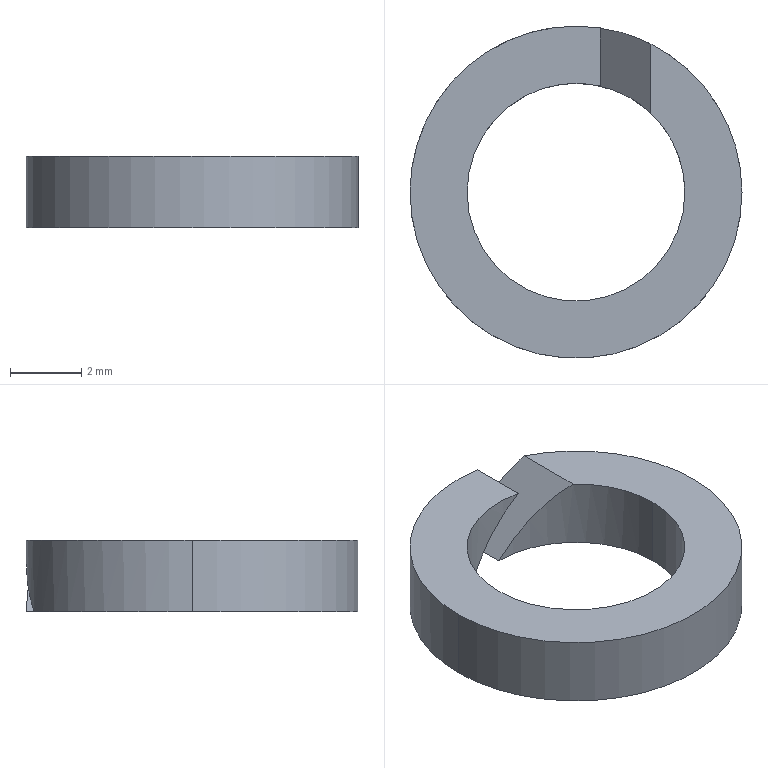Part | STEP file | 921271103 | 1 solid | 10 faces | box 9.3 x 9.3 x 2 mm | volume 72.768 mm3 | cylinder 6 | plane 4 | commonest cylinder face diameters 6.1 x3 9.3 x3
STEP:
#1=CARTESIAN_POINT('',(2.1,4.149,2.));
#2=VERTEX_POINT('',#1);
#3=CARTESIAN_POINT('',(4.65,0.,2.));
#4=VERTEX_POINT('',#3);
#5=CARTESIAN_POINT('',(0.,0.,2.));
#6=DIRECTION('',(0.,0.,-1.));
#7=DIRECTION('',(-1.,0.,0.));
#8=AXIS2_PLACEMENT_3D('',#5,#6,#7);
#9=CIRCLE('',#8,4.65);
#10=EDGE_CURVE('',#2,#4,#9,.T.);
#11=ORIENTED_EDGE('',*,*,#10,.T.);
#12=CARTESIAN_POINT('',(4.65,0.,0.));
#13=VERTEX_POINT('',#12);
#14=CARTESIAN_POINT('',(4.65,0.,2.));
#15=DIRECTION('',(0.,0.,-1.));
#16=VECTOR('',#15,1000.);
#17=LINE('',#14,#16);
#18=EDGE_CURVE('',#4,#13,#17,.T.);
#19=ORIENTED_EDGE('',*,*,#18,.T.);
#20=CARTESIAN_POINT('',(0.,4.65,0.));
#21=VERTEX_POINT('',#20);
#22=CARTESIAN_POINT('',(0.,0.,0.));
#23=DIRECTION('',(0.,0.,1.));
#24=DIRECTION('',(-1.,0.,0.));
#25=AXIS2_PLACEMENT_3D('',#22,#23,#24);
#26=CIRCLE('',#25,4.65);
#27=EDGE_CURVE('',#13,#21,#26,.T.);
#28=ORIENTED_EDGE('',*,*,#27,.T.);
#29=CARTESIAN_POINT('',(0.,4.65,0.));
#30=CARTESIAN_POINT('',(0.733,4.65,0.6981));
#31=CARTESIAN_POINT('',(1.446,4.48,1.377));
#32=CARTESIAN_POINT('',(2.1,4.149,2.));
#33=(BOUNDED_CURVE()B_SPLINE_CURVE(3,(#29,#30,#31,#32),.UNSPECIFIED.,.F.,.F.)B_SPLINE_CURVE_WITH_KNOTS((4,4),(1.571,2.039),.UNSPECIFIED.)CURVE()GEOMETRIC_REPRESENTATION_ITEM()RATIONAL_B_SPLINE_CURVE((1.,0.9818,0.9818,1.))REPRESENTATION_ITEM(''));
#34=EDGE_CURVE('',#21,#2,#33,.T.);
#35=ORIENTED_EDGE('',*,*,#34,.T.);
#36=EDGE_LOOP('',(#11,#19,#28,#35));
#37=FACE_OUTER_BOUND('',#36,.T.);
#38=CARTESIAN_POINT('',(0.,0.,2.));
#39=DIRECTION('',(0.,0.,-1.));
#40=DIRECTION('',(-1.,0.,0.));
#41=AXIS2_PLACEMENT_3D('',#38,#39,#40);
#42=CYLINDRICAL_SURFACE('',#41,4.65);
#43=ADVANCED_FACE('',(#37),#42,.T.);
#44=ORIENTED_EDGE('',*,*,#18,.F.);
#45=CARTESIAN_POINT('',(-4.65,0.,2.));
#46=VERTEX_POINT('',#45);
#47=CARTESIAN_POINT('',(0.,0.,2.));
#48=DIRECTION('',(0.,0.,-1.));
#49=DIRECTION('',(-1.,0.,0.));
#50=AXIS2_PLACEMENT_3D('',#47,#48,#49);
#51=CIRCLE('',#50,4.65);
#52=EDGE_CURVE('',#4,#46,#51,.T.);
#53=ORIENTED_EDGE('',*,*,#52,.T.);
#54=CARTESIAN_POINT('',(-4.65,0.,0.));
#55=VERTEX_POINT('',#54);
#56=CARTESIAN_POINT('',(-4.65,0.,2.));
#57=DIRECTION('',(0.,0.,-1.));
#58=VECTOR('',#57,1000.);
#59=LINE('',#56,#58);
#60=EDGE_CURVE('',#46,#55,#59,.T.);
#61=ORIENTED_EDGE('',*,*,#60,.T.);
#62=CARTESIAN_POINT('',(0.,0.,0.));
#63=DIRECTION('',(0.,0.,1.));
#64=DIRECTION('',(-1.,0.,0.));
#65=AXIS2_PLACEMENT_3D('',#62,#63,#64);
#66=CIRCLE('',#65,4.65);
#67=EDGE_CURVE('',#55,#13,#66,.T.);
#68=ORIENTED_EDGE('',*,*,#67,.T.);
#69=EDGE_LOOP('',(#44,#53,#61,#68));
#70=FACE_OUTER_BOUND('',#69,.T.);
#71=CARTESIAN_POINT('',(0.,0.,2.));
#72=DIRECTION('',(0.,0.,-1.));
#73=DIRECTION('',(-1.,0.,0.));
#74=AXIS2_PLACEMENT_3D('',#71,#72,#73);
#75=CYLINDRICAL_SURFACE('',#74,4.65);
#76=ADVANCED_FACE('',(#70),#75,.T.);
#77=CARTESIAN_POINT('',(-3.05,0.,2.));
#78=VERTEX_POINT('',#77);
#79=CARTESIAN_POINT('',(3.05,0.,2.));
#80=VERTEX_POINT('',#79);
#81=CARTESIAN_POINT('',(0.,0.,2.));
#82=DIRECTION('',(0.,0.,1.));
#83=DIRECTION('',(-1.,0.,0.));
#84=AXIS2_PLACEMENT_3D('',#81,#82,#83);
#85=CIRCLE('',#84,3.05);
#86=EDGE_CURVE('',#78,#80,#85,.T.);
#87=ORIENTED_EDGE('',*,*,#86,.T.);
#88=CARTESIAN_POINT('',(3.05,0.,0.));
#89=VERTEX_POINT('',#88);
#90=CARTESIAN_POINT('',(3.05,0.,2.));
#91=DIRECTION('',(0.,0.,-1.));
#92=VECTOR('',#91,1000.);
#93=LINE('',#90,#92);
#94=EDGE_CURVE('',#80,#89,#93,.T.);
#95=ORIENTED_EDGE('',*,*,#94,.T.);
#96=CARTESIAN_POINT('',(-3.05,0.,0.));
#97=VERTEX_POINT('',#96);
#98=CARTESIAN_POINT('',(0.,0.,0.));
#99=DIRECTION('',(0.,0.,1.));
#100=DIRECTION('',(-1.,0.,0.));
#101=AXIS2_PLACEMENT_3D('',#98,#99,#100);
#102=CIRCLE('',#101,3.05);
#103=EDGE_CURVE('',#97,#89,#102,.T.);
#104=ORIENTED_EDGE('',*,*,#103,.F.);
#105=CARTESIAN_POINT('',(-3.05,0.,2.));
#106=DIRECTION('',(0.,0.,-1.));
#107=VECTOR('',#106,1000.);
#108=LINE('',#105,#107);
#109=EDGE_CURVE('',#78,#97,#108,.T.);
#110=ORIENTED_EDGE('',*,*,#109,.F.);
#111=EDGE_LOOP('',(#87,#95,#104,#110));
#112=FACE_OUTER_BOUND('',#111,.T.);
#113=CARTESIAN_POINT('',(0.,0.,2.));
#114=DIRECTION('',(0.,0.,-1.));
#115=DIRECTION('',(-1.,0.,0.));
#116=AXIS2_PLACEMENT_3D('',#113,#114,#115);
#117=CYLINDRICAL_SURFACE('',#116,3.05);
#118=ADVANCED_FACE('',(#112),#117,.F.);
#119=CARTESIAN_POINT('',(0.6858,2.972,2.));
#120=VERTEX_POINT('',#119);
#121=CARTESIAN_POINT('',(0.,0.,2.));
#122=DIRECTION('',(0.,0.,1.));
#123=DIRECTION('',(-1.,0.,0.));
#124=AXIS2_PLACEMENT_3D('',#121,#122,#123);
#125=CIRCLE('',#124,3.05);
#126=EDGE_CURVE('',#120,#78,#125,.T.);
#127=ORIENTED_EDGE('',*,*,#126,.T.);
#128=ORIENTED_EDGE('',*,*,#109,.T.);
#129=CARTESIAN_POINT('',(-1.414,2.702,0.));
#130=VERTEX_POINT('',#129);
#131=CARTESIAN_POINT('',(0.,0.,0.));
#132=DIRECTION('',(0.,0.,1.));
#133=DIRECTION('',(-1.,0.,0.));
#134=AXIS2_PLACEMENT_3D('',#131,#132,#133);
#135=CIRCLE('',#134,3.05);
#136=EDGE_CURVE('',#130,#97,#135,.T.);
#137=ORIENTED_EDGE('',*,*,#136,.F.);
#138=CARTESIAN_POINT('',(0.6858,2.972,2.));
#139=CARTESIAN_POINT('',(-0.03162,3.137,1.317));
#140=CARTESIAN_POINT('',(-0.7619,3.044,0.6213));
#141=CARTESIAN_POINT('',(-1.414,2.702,0.));
#142=(BOUNDED_CURVE()B_SPLINE_CURVE(3,(#138,#139,#140,#141),.UNSPECIFIED.,.F.,.F.)B_SPLINE_CURVE_WITH_KNOTS((4,4),(4.486,5.195),.UNSPECIFIED.)CURVE()GEOMETRIC_REPRESENTATION_ITEM()RATIONAL_B_SPLINE_CURVE((1.,0.9586,0.9586,1.))REPRESENTATION_ITEM(''));
#143=EDGE_CURVE('',#120,#130,#142,.T.);
#144=ORIENTED_EDGE('',*,*,#143,.F.);
#145=EDGE_LOOP('',(#127,#128,#137,#144));
#146=FACE_OUTER_BOUND('',#145,.T.);
#147=CARTESIAN_POINT('',(0.,0.,2.));
#148=DIRECTION('',(0.,0.,-1.));
#149=DIRECTION('',(-1.,0.,0.));
#150=AXIS2_PLACEMENT_3D('',#147,#148,#149);
#151=CYLINDRICAL_SURFACE('',#150,3.05);
#152=ADVANCED_FACE('',(#146),#151,.F.);
#153=ORIENTED_EDGE('',*,*,#60,.F.);
#154=CARTESIAN_POINT('',(0.6858,4.599,2.));
#155=VERTEX_POINT('',#154);
#156=CARTESIAN_POINT('',(0.,0.,2.));
#157=DIRECTION('',(0.,0.,-1.));
#158=DIRECTION('',(-1.,0.,0.));
#159=AXIS2_PLACEMENT_3D('',#156,#157,#158);
#160=CIRCLE('',#159,4.65);
#161=EDGE_CURVE('',#46,#155,#160,.T.);
#162=ORIENTED_EDGE('',*,*,#161,.T.);
#163=CARTESIAN_POINT('',(-1.414,4.43,0.));
#164=VERTEX_POINT('',#163);
#165=CARTESIAN_POINT('',(0.6858,4.599,2.));
#166=CARTESIAN_POINT('',(-0.02106,4.705,1.327));
#167=CARTESIAN_POINT('',(-0.7334,4.647,0.6484));
#168=CARTESIAN_POINT('',(-1.414,4.43,0.));
#169=(BOUNDED_CURVE()B_SPLINE_CURVE(3,(#165,#166,#167,#168),.UNSPECIFIED.,.F.,.F.)B_SPLINE_CURVE_WITH_KNOTS((4,4),(4.564,5.021),.UNSPECIFIED.)CURVE()GEOMETRIC_REPRESENTATION_ITEM()RATIONAL_B_SPLINE_CURVE((1.,0.9827,0.9827,1.))REPRESENTATION_ITEM(''));
#170=EDGE_CURVE('',#155,#164,#169,.T.);
#171=ORIENTED_EDGE('',*,*,#170,.T.);
#172=CARTESIAN_POINT('',(0.,0.,0.));
#173=DIRECTION('',(0.,0.,1.));
#174=DIRECTION('',(-1.,0.,0.));
#175=AXIS2_PLACEMENT_3D('',#172,#173,#174);
#176=CIRCLE('',#175,4.65);
#177=EDGE_CURVE('',#164,#55,#176,.T.);
#178=ORIENTED_EDGE('',*,*,#177,.T.);
#179=EDGE_LOOP('',(#153,#162,#171,#178));
#180=FACE_OUTER_BOUND('',#179,.T.);
#181=CARTESIAN_POINT('',(0.,0.,2.));
#182=DIRECTION('',(0.,0.,-1.));
#183=DIRECTION('',(-1.,0.,0.));
#184=AXIS2_PLACEMENT_3D('',#181,#182,#183);
#185=CYLINDRICAL_SURFACE('',#184,4.65);
#186=ADVANCED_FACE('',(#180),#185,.T.);
#187=CARTESIAN_POINT('',(-1.414,5.115,0.));
#188=DIRECTION('',(0.,1.,0.));
#189=VECTOR('',#188,1000.);
#190=LINE('',#187,#189);
#191=EDGE_CURVE('',#130,#164,#190,.T.);
#192=ORIENTED_EDGE('',*,*,#191,.T.);
#193=ORIENTED_EDGE('',*,*,#170,.F.);
#194=CARTESIAN_POINT('',(0.6858,5.115,2.));
#195=DIRECTION('',(0.,-1.,0.));
#196=VECTOR('',#195,1000.);
#197=LINE('',#194,#196);
#198=EDGE_CURVE('',#155,#120,#197,.T.);
#199=ORIENTED_EDGE('',*,*,#198,.T.);
#200=ORIENTED_EDGE('',*,*,#143,.T.);
#201=EDGE_LOOP('',(#192,#193,#199,#200));
#202=FACE_OUTER_BOUND('',#201,.T.);
#203=CARTESIAN_POINT('',(-1.414,5.115,0.));
#204=DIRECTION('',(0.6897,0.,-0.7241));
#205=DIRECTION('',(-0.7241,0.,-0.6897));
#206=AXIS2_PLACEMENT_3D('',#203,#204,#205);
#207=PLANE('',#206);
#208=ADVANCED_FACE('',(#202),#207,.T.);
#209=ORIENTED_EDGE('',*,*,#126,.F.);
#210=ORIENTED_EDGE('',*,*,#198,.F.);
#211=ORIENTED_EDGE('',*,*,#161,.F.);
#212=ORIENTED_EDGE('',*,*,#52,.F.);
#213=ORIENTED_EDGE('',*,*,#10,.F.);
#214=CARTESIAN_POINT('',(2.1,2.212,2.));
#215=VERTEX_POINT('',#214);
#216=CARTESIAN_POINT('',(2.1,0.,2.));
#217=DIRECTION('',(0.,1.,0.));
#218=VECTOR('',#217,1000.);
#219=LINE('',#216,#218);
#220=EDGE_CURVE('',#215,#2,#219,.T.);
#221=ORIENTED_EDGE('',*,*,#220,.F.);
#222=CARTESIAN_POINT('',(0.,0.,2.));
#223=DIRECTION('',(0.,0.,1.));
#224=DIRECTION('',(-1.,0.,0.));
#225=AXIS2_PLACEMENT_3D('',#222,#223,#224);
#226=CIRCLE('',#225,3.05);
#227=EDGE_CURVE('',#80,#215,#226,.T.);
#228=ORIENTED_EDGE('',*,*,#227,.F.);
#229=ORIENTED_EDGE('',*,*,#86,.F.);
#230=EDGE_LOOP('',(#209,#210,#211,#212,#213,#221,#228,#229));
#231=FACE_OUTER_BOUND('',#230,.T.);
#232=CARTESIAN_POINT('',(0.,0.,2.));
#233=DIRECTION('',(0.,0.,-1.));
#234=DIRECTION('',(-1.,0.,0.));
#235=AXIS2_PLACEMENT_3D('',#232,#233,#234);
#236=PLANE('',#235);
#237=ADVANCED_FACE('',(#231),#236,.F.);
#238=ORIENTED_EDGE('',*,*,#220,.T.);
#239=ORIENTED_EDGE('',*,*,#34,.F.);
#240=CARTESIAN_POINT('',(0.,3.05,0.));
#241=VERTEX_POINT('',#240);
#242=CARTESIAN_POINT('',(0.,5.115,0.));
#243=DIRECTION('',(0.,-1.,0.));
#244=VECTOR('',#243,1000.);
#245=LINE('',#242,#244);
#246=EDGE_CURVE('',#21,#241,#245,.T.);
#247=ORIENTED_EDGE('',*,*,#246,.T.);
#248=CARTESIAN_POINT('',(0.,3.05,0.));
#249=CARTESIAN_POINT('',(0.7913,3.05,0.7536));
#250=CARTESIAN_POINT('',(1.526,2.757,1.453));
#251=CARTESIAN_POINT('',(2.1,2.212,2.));
#252=(BOUNDED_CURVE()B_SPLINE_CURVE(3,(#248,#249,#250,#251),.UNSPECIFIED.,.F.,.F.)B_SPLINE_CURVE_WITH_KNOTS((4,4),(1.571,2.33),.UNSPECIFIED.)CURVE()GEOMETRIC_REPRESENTATION_ITEM()RATIONAL_B_SPLINE_CURVE((1.,0.9525,0.9525,1.))REPRESENTATION_ITEM(''));
#253=EDGE_CURVE('',#241,#215,#252,.T.);
#254=ORIENTED_EDGE('',*,*,#253,.T.);
#255=EDGE_LOOP('',(#238,#239,#247,#254));
#256=FACE_OUTER_BOUND('',#255,.T.);
#257=CARTESIAN_POINT('',(2.1,5.115,2.));
#258=DIRECTION('',(-0.6897,0.,0.7241));
#259=DIRECTION('',(0.7241,0.,0.6897));
#260=AXIS2_PLACEMENT_3D('',#257,#258,#259);
#261=PLANE('',#260);
#262=ADVANCED_FACE('',(#256),#261,.T.);
#263=ORIENTED_EDGE('',*,*,#177,.F.);
#264=ORIENTED_EDGE('',*,*,#191,.F.);
#265=ORIENTED_EDGE('',*,*,#136,.T.);
#266=ORIENTED_EDGE('',*,*,#103,.T.);
#267=CARTESIAN_POINT('',(0.,0.,0.));
#268=DIRECTION('',(0.,0.,1.));
#269=DIRECTION('',(-1.,0.,0.));
#270=AXIS2_PLACEMENT_3D('',#267,#268,#269);
#271=CIRCLE('',#270,3.05);
#272=EDGE_CURVE('',#89,#241,#271,.T.);
#273=ORIENTED_EDGE('',*,*,#272,.T.);
#274=ORIENTED_EDGE('',*,*,#246,.F.);
#275=ORIENTED_EDGE('',*,*,#27,.F.);
#276=ORIENTED_EDGE('',*,*,#67,.F.);
#277=EDGE_LOOP('',(#263,#264,#265,#266,#273,#274,#275,#276));
#278=FACE_OUTER_BOUND('',#277,.T.);
#279=CARTESIAN_POINT('',(0.,0.,0.));
#280=DIRECTION('',(0.,0.,-1.));
#281=DIRECTION('',(-1.,0.,0.));
#282=AXIS2_PLACEMENT_3D('',#279,#280,#281);
#283=PLANE('',#282);
#284=ADVANCED_FACE('',(#278),#283,.T.);
#285=ORIENTED_EDGE('',*,*,#94,.F.);
#286=ORIENTED_EDGE('',*,*,#227,.T.);
#287=ORIENTED_EDGE('',*,*,#253,.F.);
#288=ORIENTED_EDGE('',*,*,#272,.F.);
#289=EDGE_LOOP('',(#285,#286,#287,#288));
#290=FACE_OUTER_BOUND('',#289,.T.);
#291=CARTESIAN_POINT('',(0.,0.,2.));
#292=DIRECTION('',(0.,0.,-1.));
#293=DIRECTION('',(-1.,0.,0.));
#294=AXIS2_PLACEMENT_3D('',#291,#292,#293);
#295=CYLINDRICAL_SURFACE('',#294,3.05);
#296=ADVANCED_FACE('',(#290),#295,.F.);
#297=CLOSED_SHELL('',(#43,#76,#118,#152,#186,#208,#237,#262,#284,#296));
#298=MANIFOLD_SOLID_BREP('',#297);
#299=CARTESIAN_POINT('',(0.,0.,0.));
#300=DIRECTION('',(0.,0.,1.));
#301=DIRECTION('',(1.,0.,0.));
#302=AXIS2_PLACEMENT_3D('',#299,#300,#301);
#303=(LENGTH_UNIT()NAMED_UNIT(*)SI_UNIT(.MILLI.,.METRE.));
#304=UNCERTAINTY_MEASURE_WITH_UNIT(LENGTH_MEASURE(0.00001),#303,'','');
#305=(NAMED_UNIT(*)PLANE_ANGLE_UNIT()SI_UNIT($,.RADIAN.));
#306=(NAMED_UNIT(*)SI_UNIT($,.STERADIAN.)SOLID_ANGLE_UNIT());
#307=(GEOMETRIC_REPRESENTATION_CONTEXT(3)GLOBAL_UNCERTAINTY_ASSIGNED_CONTEXT((#304))GLOBAL_UNIT_ASSIGNED_CONTEXT((#303,#305,#306))REPRESENTATION_CONTEXT('',''));
#308=ADVANCED_BREP_SHAPE_REPRESENTATION('',(#298,#302),#307);